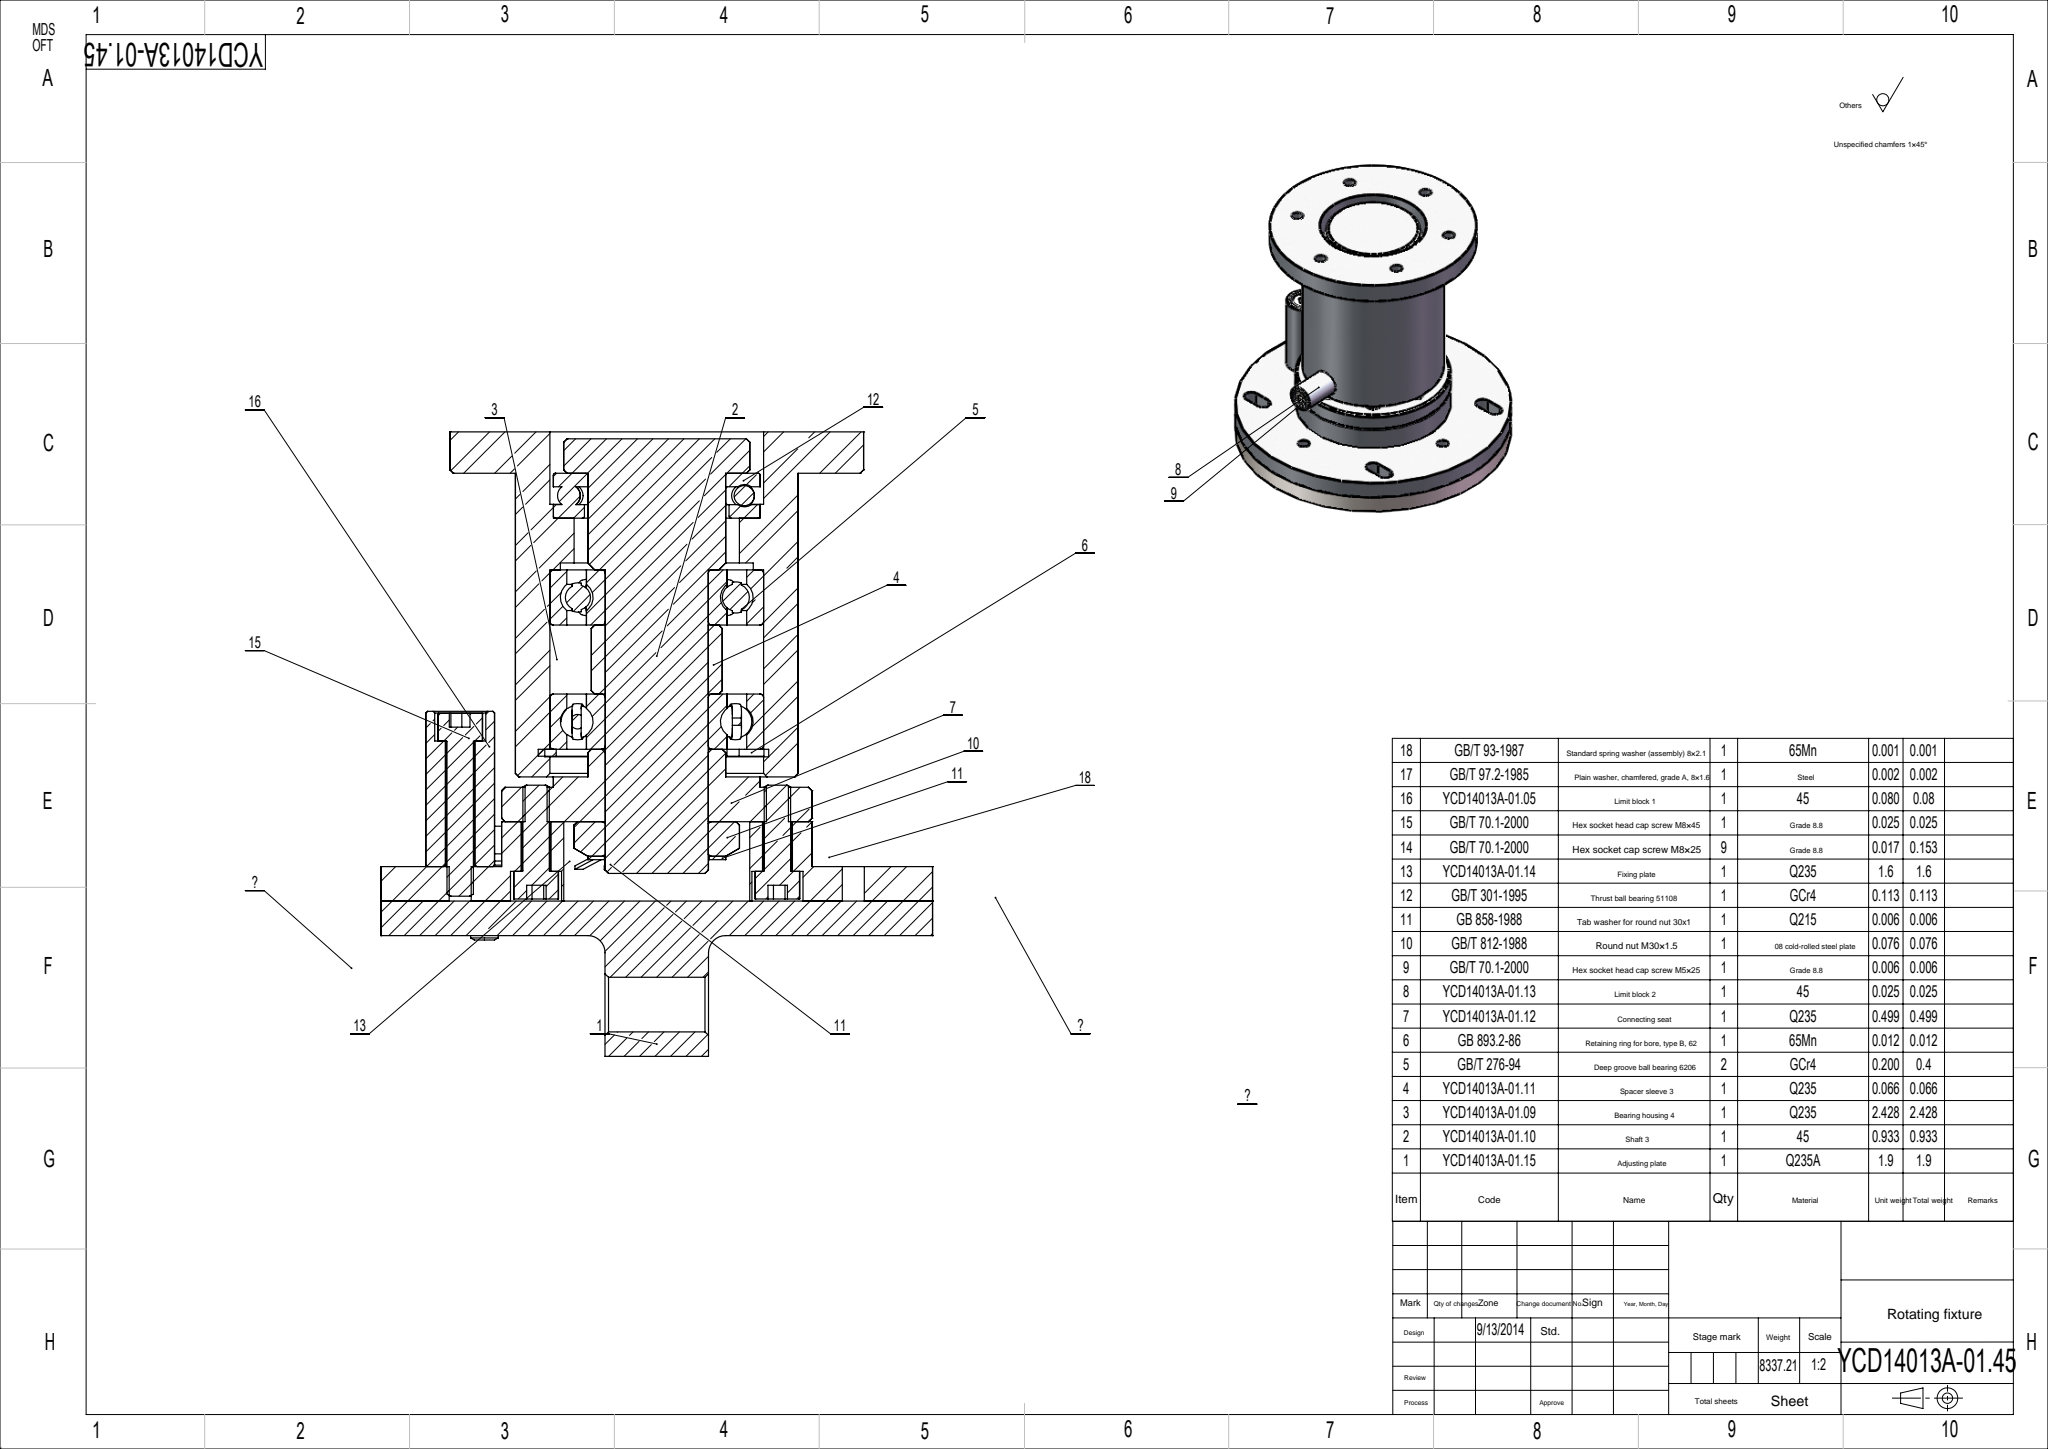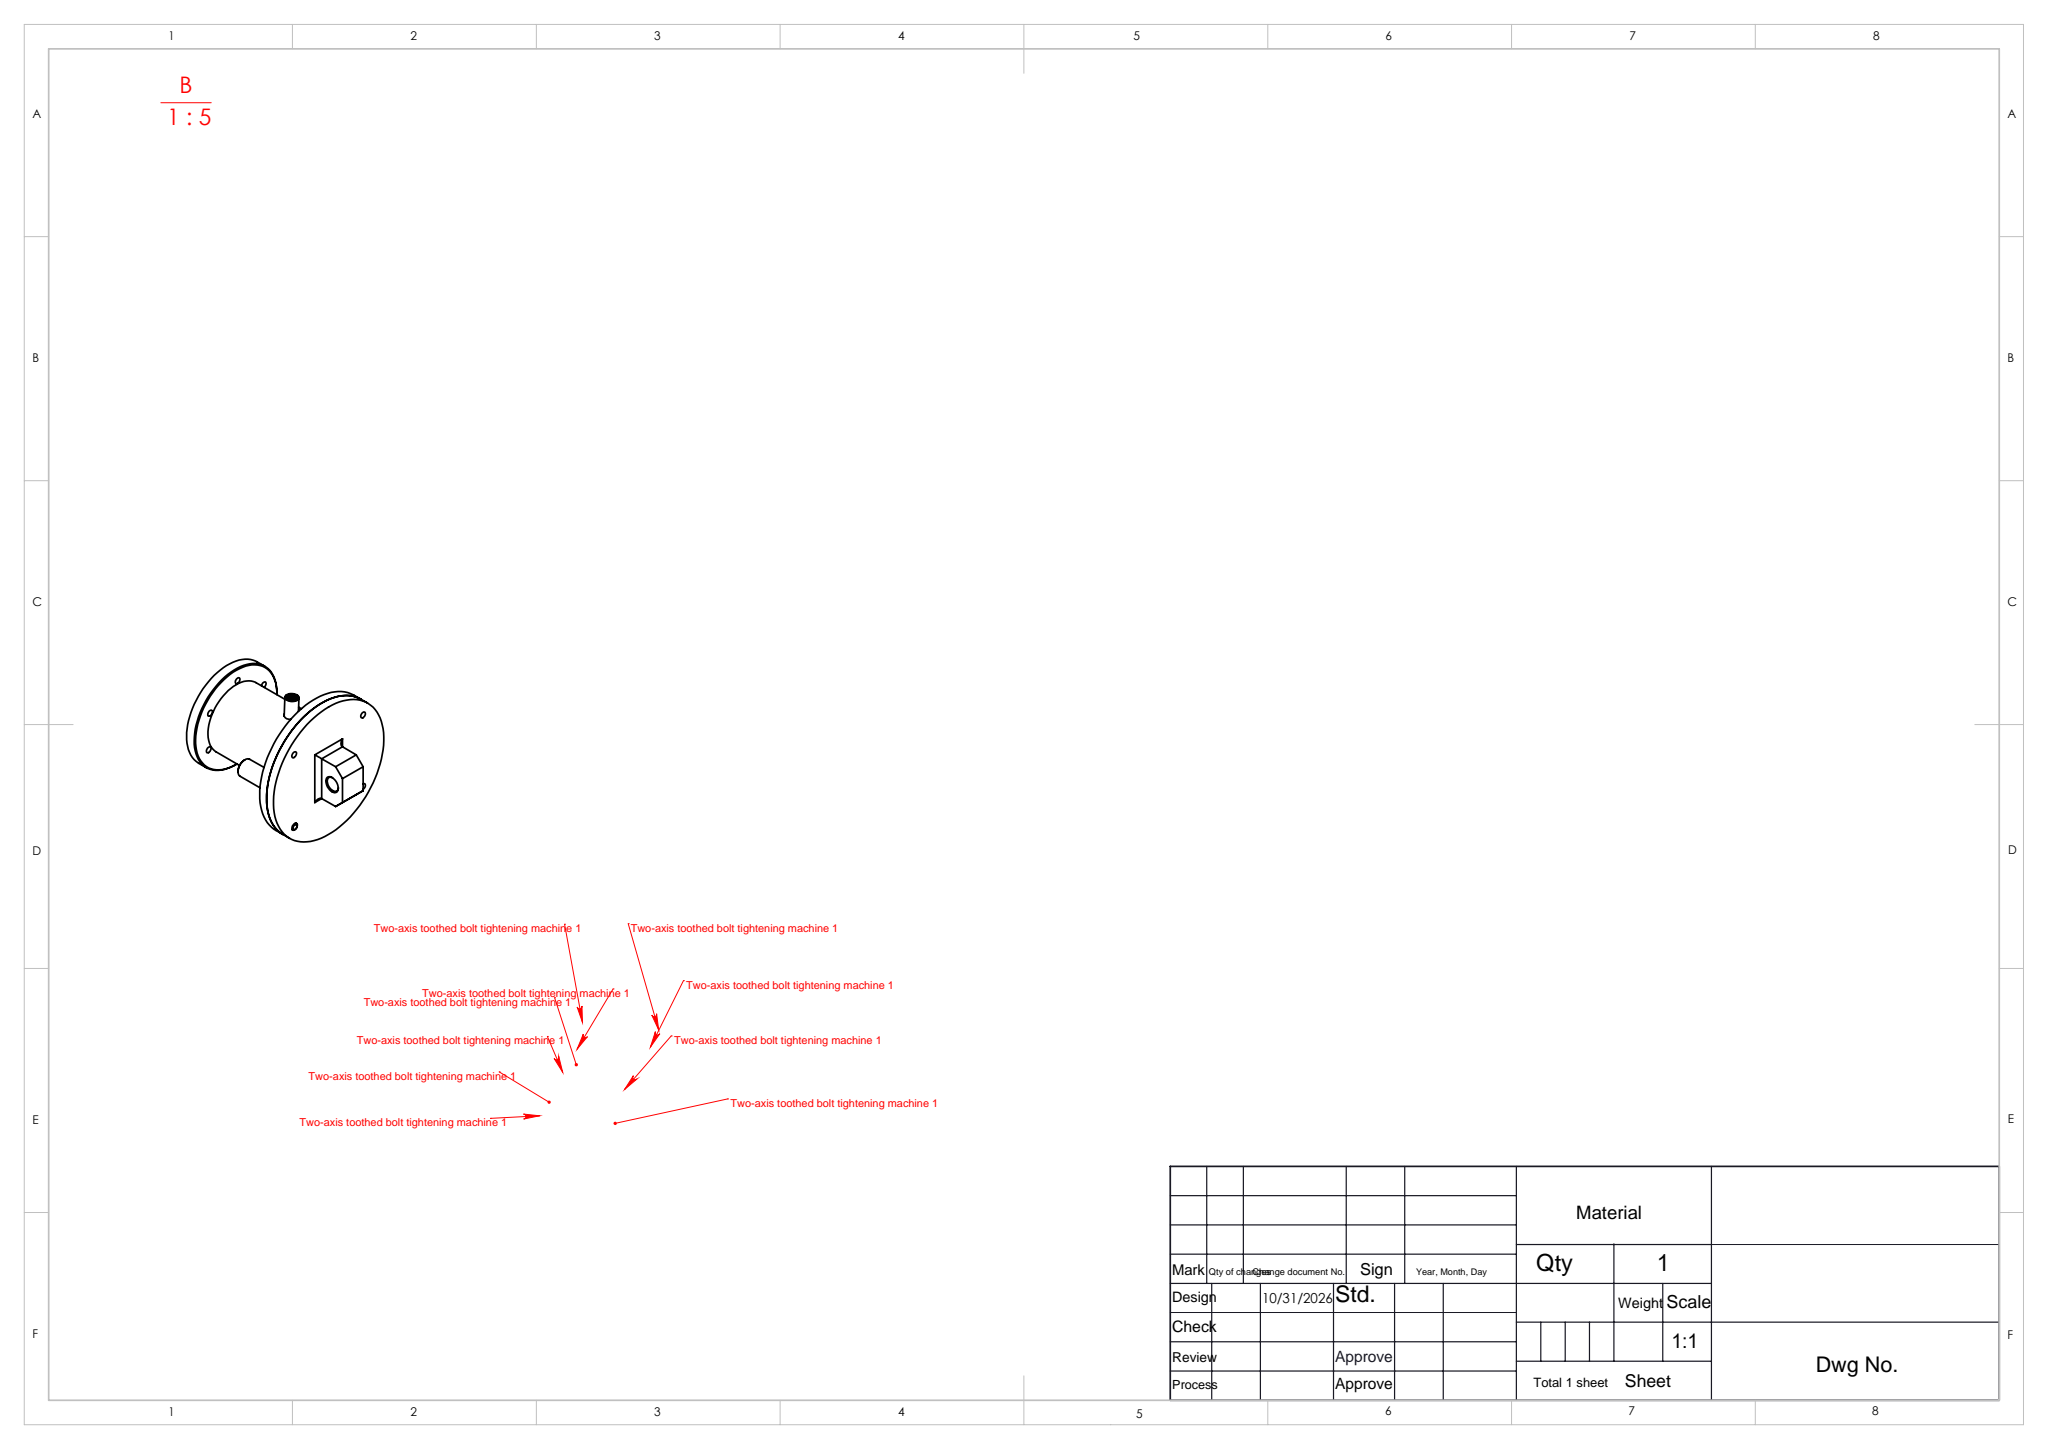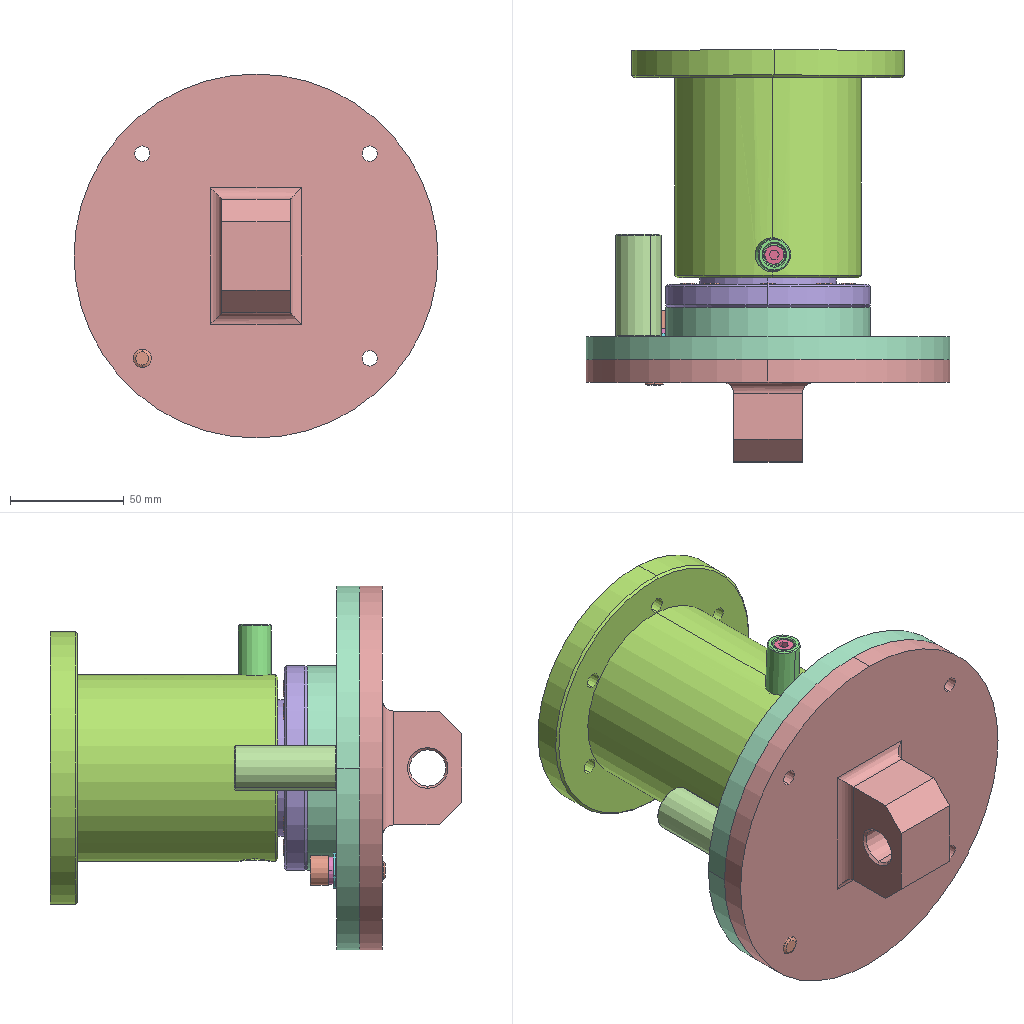Assembly | SolidWorks | 20 different items | 29 placed | box 160 x 181 x 160 mm
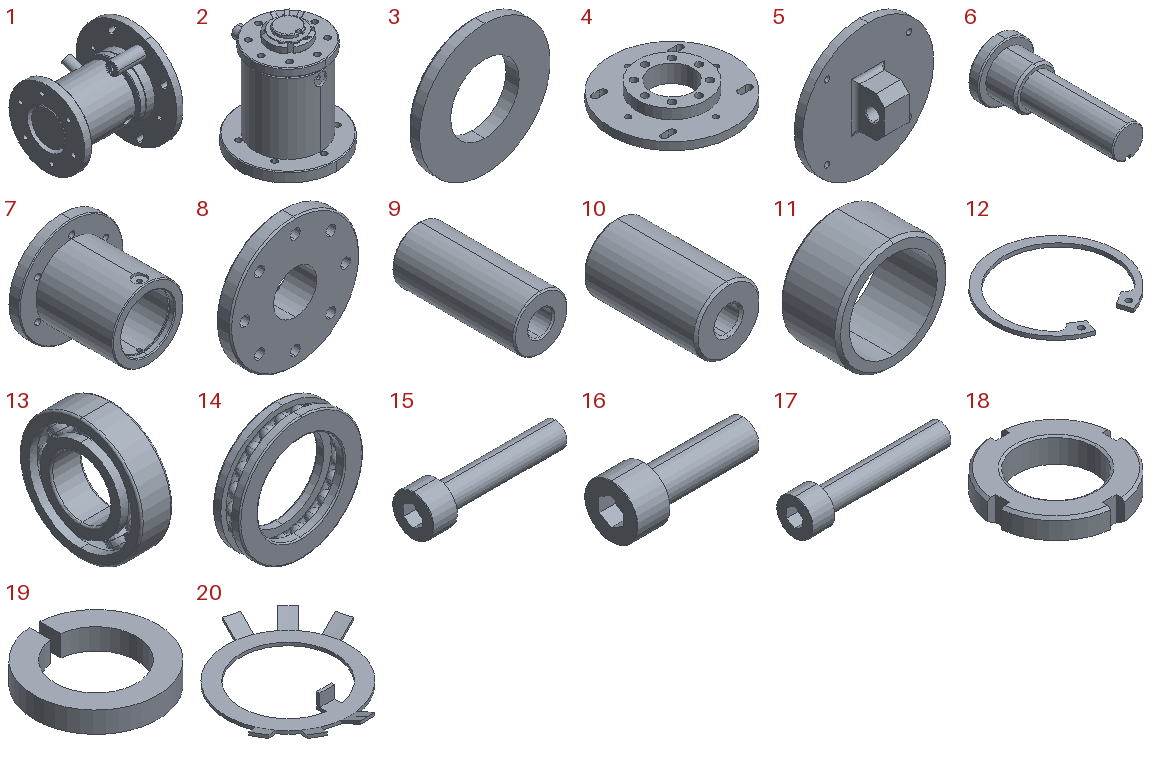Parts list (item | name | quantity | parent item | size | volume | features):
1 | (subassembly) | x1 | - | 136 x 160 x 160 mm | 819562 mm3 | features ReferencePattern 7, LocalCirPattern 1
2 | (subassembly) | x1 | in 1 | 120 x 123 x 128 mm | 584143 mm3 | -
3 | - | x1 | - | 16 x 1.6 x 16 mm | 229.077 mm3 | features Revolution 1
4 | - | x1 | in 1 | 160 x 160 x 23 mm | 204439 mm3 | features ICE 3, CirPattern 2, HoleWzd 2, Extrusion 1
5 | - | x1 | - | 160 x 45 x 160 mm | 243931 mm3 | features ICE 3, Chamfer 2, Fillet 2, Extrusion 1, HoleWzd 1
6 | - | x1 | in 2 | 54 x 126 x 54 mm | 119564 mm3 | features ICE 4, Chamfer 2, Extrusion 1
7 | - | x1 | in 2 | 120 x 100 x 120 mm | 311261 mm3 | features ICE 7, Chamfer 2, HoleWzd 2, CirPattern 1, Extrusion 1, MirrorPattern 1, RevCut 1
8 | - | x1 | in 2 | 90 x 21 x 90 mm | 64013 mm3 | features ICE 3, Chamfer 2, CirPattern 2, HoleWzd 2, Extrusion 1
9 | - | x1 | in 1 | 20 x 45 x 20 mm | 10277 mm3 | features Chamfer 1, Extrusion 1, HoleWzd 1
10 | - | x1 | in 2 | 14.5 x 25 x 14.5 mm | 3205 mm3 | features Chamfer 1, Extrusion 1, HoleWzd 1
11 | - | x1 | in 2 | 38 x 20 x 38 mm | 8428 mm3 | features Chamfer 1, Extrusion 1
12 | - | x1 | in 2 | 66.2 x 64.58 x 2 mm | 1598 mm3 | features Extrusion 1
13 | - | x2 | in 2 | 16 x 62 x 62 mm | 25311 mm3 | features Revolution 5, CirPattern 2, RevCut 2
14 | - | x1 | in 2 | 60 x 13 x 60 mm | 14302 mm3 | features Revolution 3, CirPattern 1, Fillet 1
15 | - | x1 | in 2 | 30 x 8.5 x 8.5 mm | 738.642 mm3 | features BlendCut 1, Cut 1, Fillet 1, LPattern 1, RevCut 1, Revolution 1
16 | - | x9 | in 1 | 33 x 13 x 13 mm | 2189 mm3 | features BlendCut 1, Cut 1, Fillet 1, LPattern 1, RevCut 1, Revolution 1
17 | - | x1 | in 1 | 53 x 13 x 13 mm | 3194 mm3 | features BlendCut 1, Cut 1, Fillet 1, LPattern 1, RevCut 1, Revolution 1
18 | - | x1 | in 2 | 47.706 x 47.706 x 10 mm | 9680 mm3 | features Chamfer 3, CirPattern 1, Cut 1, Extrusion 1
19 | - | x1 | - | 12.277 x 12.254 x 2.1 mm | 135.755 mm3 | features Extrusion 1
20 | - | x1 | in 2 | 49.249 x 51.517 x 5 mm | 732.706 mm3 | features Boss 1, Cut 1, Revolution 1
Mates (type | each side: item.copy, entity, surface, feature):
In the top assembly
Coincident | 5.1 face plane Boss-Extrude1 | 4.1 face plane Boss-Extrude2
Coincident | 5.1 plane | 4.1 plane | 2 times
Concentric | 5.1 face cylinder M8 Tapped Hole1 | 16.1 face cylinder Base-Revolve
Concentric | 16.1 face cylinder Base-Revolve | 3.1 face cylinder Base-Revolve
Concentric | 16.1 face cylinder Base-Revolve | 19.1 face cylinder Extrude1
Coincident | 16.1 face plane Base-Revolve | 19.1 face plane Extrude1
Coincident | 3.1 face plane Base-Revolve | 19.1 face plane Extrude1
Coincident | 4.1 face plane Boss-Extrude2 | 3.1 face plane Base-Revolve
In subassembly 1
Coincident | 8.1 face plane Boss-Extrude3 | 4.2 face plane Boss-Extrude1
Concentric | 8.1 face cylinder Boss-Extrude3 | 4.2 face cylinder Boss-Extrude1
Coincident | 4.2 face plane Boss-Extrude2 | 9.1 face plane Boss-Extrude1
Coincident | 17.1 face plane Base-Revolve | 9.1 face plane CBORE for M8 Hex Socket Head Cap Screw1
Concentric | 17.1 face cylinder Base-Revolve | 9.1 face cylinder CBORE for M8 Hex Socket Head Cap Screw1
Concentric | 4.2 face cylinder CirPattern1 | 17.1 face cylinder Base-Revolve
Coincident | 4.2 face plane CirPattern2 | 16.1 face plane Base-Revolve
Concentric | 4.2 face cylinder CirPattern2 | 16.1 face cylinder Base-Revolve
Concentric | 8.1 face cylinder CirPattern2 | 16.2 face cylinder Base-Revolve
In subassembly 2
Concentric | 6.1 face cylinder Boss-Extrude3 | 11.1 face cylinder Boss-Extrude1
Concentric | 6.1 face cylinder Boss-Extrude3 | 8.2 face cylinder Cut-Extrude1
Concentric | 7.1 face cylinder Boss-Extrude1 | 6.1 face cylinder Boss-Extrude2
Coincident | 7.1 face plane Cut-Revolve1 | 10.1 face plane Boss-Extrude1
Concentric | 7.1 face cylinder Cut-Revolve1 | 10.1 face cylinder Boss-Extrude1
Coincident | 7.1 plane | 2.1 plane
Coincident | 7.1 face plane Boss-Extrude1 | 2.1 plane
Coincident | 10.1 face plane Hole Size by Hex Socket Screw Type1 | 15.1 face plane Base-Revolve
Concentric | 10.1 face cylinder Hole Size by Hex Socket Screw Type1 | 15.1 face cylinder Base-Revolve
Coincident | 8.2 face plane Boss-Extrude3 | 18.1 face plane Base-Extrude
Concentric | 6.1 face cylinder Boss-Extrude3 | 18.1 face cylinder Base-Extrude
Coincident | 18.1 face plane Base-Extrude | 20.1 face plane Base-Revolve
Concentric | 6.1 face cylinder Boss-Extrude3 | 20.1 face cylinder Cut-Extrude2
Coincident | 6.1 face plane Cut-Extrude2 | 20.1 face plane Cut-Extrude2
Coincident | 6.1 face plane Boss-Extrude1 | 13.1 face plane Boss-Revolve4
Concentric | 6.1 face cylinder Boss-Extrude3 | 13.1 face cylinder Boss-Revolve4
Coincident | 11.1 face plane Boss-Extrude1 | 13.1 face plane Boss-Revolve4
Concentric | 6.1 face cylinder Boss-Extrude3 | 13.2 face cylinder Boss-Revolve4
Coincident | 11.1 face plane Boss-Extrude1 | 13.2 face plane Boss-Revolve4
Concentric | 7.1 face cylinder Cut-Extrude8 | 14.1 face cylinder Base-Revolve
Coincident | 7.1 face plane Cut-Extrude2 | 14.1 face plane Base-Revolve
Coincident | 13.2 face plane Boss-Revolve4 | 8.2 face plane Boss-Extrude1
Concentric | 12.1 face cylinder Base-Extrude | 8.2 face cylinder Boss-Extrude1
Coincident | 13.2 face plane Boss-Revolve3 | 12.1 face plane Base-Extrude